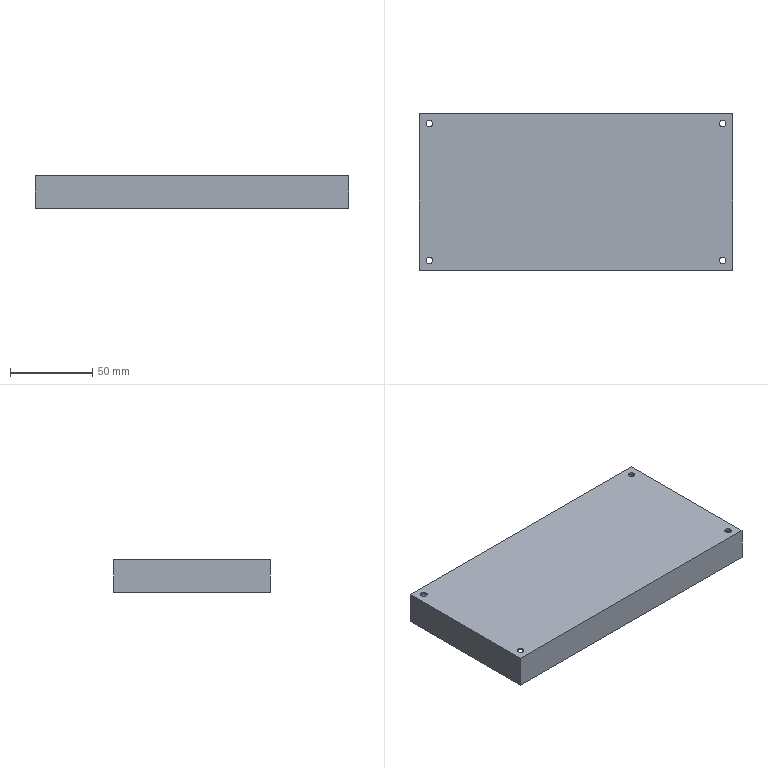Part | SolidWorks | features ICE 9, Extrusion 1, Shell 1 | 1 solid | 19 faces | box 190 x 95 x 20 mm | volume 28754 mm3 | plane 11 | cylinder 8 | commonest cylinder face diameters 4 x8
STEP:
#1=CARTESIAN_POINT('',(154.139,-3.375,19.));
#2=VERTEX_POINT('',#1);
#3=CARTESIAN_POINT('',(158.139,-3.375,19.));
#4=VERTEX_POINT('',#3);
#5=CARTESIAN_POINT('',(156.139,-3.375,19.));
#6=DIRECTION('',(0.,0.,1.));
#7=DIRECTION('',(1.,0.,0.));
#8=AXIS2_PLACEMENT_3D('',#5,#6,#7);
#9=CIRCLE('',#8,2.);
#10=EDGE_CURVE('',#2,#4,#9,.T.);
#11=ORIENTED_EDGE('',*,*,#10,.F.);
#12=CARTESIAN_POINT('',(154.139,-3.375,20.));
#13=VERTEX_POINT('',#12);
#14=CARTESIAN_POINT('',(154.139,-3.375,19.));
#15=DIRECTION('',(0.,0.,1.));
#16=VECTOR('',#15,1000.);
#17=LINE('',#14,#16);
#18=EDGE_CURVE('',#2,#13,#17,.T.);
#19=ORIENTED_EDGE('',*,*,#18,.T.);
#20=CARTESIAN_POINT('',(158.139,-3.375,20.));
#21=VERTEX_POINT('',#20);
#22=CARTESIAN_POINT('',(156.139,-3.375,20.));
#23=DIRECTION('',(0.,0.,1.));
#24=DIRECTION('',(1.,0.,0.));
#25=AXIS2_PLACEMENT_3D('',#22,#23,#24);
#26=CIRCLE('',#25,2.);
#27=EDGE_CURVE('',#13,#21,#26,.T.);
#28=ORIENTED_EDGE('',*,*,#27,.T.);
#29=CARTESIAN_POINT('',(158.139,-3.375,19.));
#30=DIRECTION('',(0.,0.,1.));
#31=VECTOR('',#30,1000.);
#32=LINE('',#29,#31);
#33=EDGE_CURVE('',#4,#21,#32,.T.);
#34=ORIENTED_EDGE('',*,*,#33,.F.);
#35=EDGE_LOOP('',(#11,#19,#28,#34));
#36=FACE_OUTER_BOUND('',#35,.T.);
#37=CARTESIAN_POINT('',(156.139,-3.375,19.));
#38=DIRECTION('',(0.,0.,1.));
#39=DIRECTION('',(1.,0.,0.));
#40=AXIS2_PLACEMENT_3D('',#37,#38,#39);
#41=CYLINDRICAL_SURFACE('',#40,2.);
#42=ADVANCED_FACE('',(#36),#41,.F.);
#43=CARTESIAN_POINT('',(154.139,79.625,19.));
#44=VERTEX_POINT('',#43);
#45=CARTESIAN_POINT('',(158.139,79.625,19.));
#46=VERTEX_POINT('',#45);
#47=CARTESIAN_POINT('',(156.139,79.625,19.));
#48=DIRECTION('',(0.,0.,1.));
#49=DIRECTION('',(1.,0.,0.));
#50=AXIS2_PLACEMENT_3D('',#47,#48,#49);
#51=CIRCLE('',#50,2.);
#52=EDGE_CURVE('',#44,#46,#51,.T.);
#53=ORIENTED_EDGE('',*,*,#52,.F.);
#54=CARTESIAN_POINT('',(154.139,79.625,20.));
#55=VERTEX_POINT('',#54);
#56=CARTESIAN_POINT('',(154.139,79.625,19.));
#57=DIRECTION('',(0.,0.,1.));
#58=VECTOR('',#57,1000.);
#59=LINE('',#56,#58);
#60=EDGE_CURVE('',#44,#55,#59,.T.);
#61=ORIENTED_EDGE('',*,*,#60,.T.);
#62=CARTESIAN_POINT('',(158.139,79.625,20.));
#63=VERTEX_POINT('',#62);
#64=CARTESIAN_POINT('',(156.139,79.625,20.));
#65=DIRECTION('',(0.,0.,1.));
#66=DIRECTION('',(1.,0.,0.));
#67=AXIS2_PLACEMENT_3D('',#64,#65,#66);
#68=CIRCLE('',#67,2.);
#69=EDGE_CURVE('',#55,#63,#68,.T.);
#70=ORIENTED_EDGE('',*,*,#69,.T.);
#71=CARTESIAN_POINT('',(158.139,79.625,19.));
#72=DIRECTION('',(0.,0.,1.));
#73=VECTOR('',#72,1000.);
#74=LINE('',#71,#73);
#75=EDGE_CURVE('',#46,#63,#74,.T.);
#76=ORIENTED_EDGE('',*,*,#75,.F.);
#77=EDGE_LOOP('',(#53,#61,#70,#76));
#78=FACE_OUTER_BOUND('',#77,.T.);
#79=CARTESIAN_POINT('',(156.139,79.625,19.));
#80=DIRECTION('',(0.,0.,1.));
#81=DIRECTION('',(1.,0.,0.));
#82=AXIS2_PLACEMENT_3D('',#79,#80,#81);
#83=CYLINDRICAL_SURFACE('',#82,2.);
#84=ADVANCED_FACE('',(#78),#83,.F.);
#85=CARTESIAN_POINT('',(-23.861,79.625,19.));
#86=VERTEX_POINT('',#85);
#87=CARTESIAN_POINT('',(-19.861,79.625,19.));
#88=VERTEX_POINT('',#87);
#89=CARTESIAN_POINT('',(-21.861,79.625,19.));
#90=DIRECTION('',(0.,0.,1.));
#91=DIRECTION('',(1.,0.,0.));
#92=AXIS2_PLACEMENT_3D('',#89,#90,#91);
#93=CIRCLE('',#92,2.);
#94=EDGE_CURVE('',#86,#88,#93,.T.);
#95=ORIENTED_EDGE('',*,*,#94,.F.);
#96=CARTESIAN_POINT('',(-23.861,79.625,20.));
#97=VERTEX_POINT('',#96);
#98=CARTESIAN_POINT('',(-23.861,79.625,19.));
#99=DIRECTION('',(0.,0.,1.));
#100=VECTOR('',#99,1000.);
#101=LINE('',#98,#100);
#102=EDGE_CURVE('',#86,#97,#101,.T.);
#103=ORIENTED_EDGE('',*,*,#102,.T.);
#104=CARTESIAN_POINT('',(-19.861,79.625,20.));
#105=VERTEX_POINT('',#104);
#106=CARTESIAN_POINT('',(-21.861,79.625,20.));
#107=DIRECTION('',(0.,0.,1.));
#108=DIRECTION('',(1.,0.,0.));
#109=AXIS2_PLACEMENT_3D('',#106,#107,#108);
#110=CIRCLE('',#109,2.);
#111=EDGE_CURVE('',#97,#105,#110,.T.);
#112=ORIENTED_EDGE('',*,*,#111,.T.);
#113=CARTESIAN_POINT('',(-19.861,79.625,19.));
#114=DIRECTION('',(0.,0.,1.));
#115=VECTOR('',#114,1000.);
#116=LINE('',#113,#115);
#117=EDGE_CURVE('',#88,#105,#116,.T.);
#118=ORIENTED_EDGE('',*,*,#117,.F.);
#119=EDGE_LOOP('',(#95,#103,#112,#118));
#120=FACE_OUTER_BOUND('',#119,.T.);
#121=CARTESIAN_POINT('',(-21.861,79.625,19.));
#122=DIRECTION('',(0.,0.,1.));
#123=DIRECTION('',(1.,0.,0.));
#124=AXIS2_PLACEMENT_3D('',#121,#122,#123);
#125=CYLINDRICAL_SURFACE('',#124,2.);
#126=ADVANCED_FACE('',(#120),#125,.F.);
#127=CARTESIAN_POINT('',(-23.861,-3.375,19.));
#128=VERTEX_POINT('',#127);
#129=CARTESIAN_POINT('',(-19.861,-3.375,19.));
#130=VERTEX_POINT('',#129);
#131=CARTESIAN_POINT('',(-21.861,-3.375,19.));
#132=DIRECTION('',(0.,0.,1.));
#133=DIRECTION('',(1.,0.,0.));
#134=AXIS2_PLACEMENT_3D('',#131,#132,#133);
#135=CIRCLE('',#134,2.);
#136=EDGE_CURVE('',#128,#130,#135,.T.);
#137=ORIENTED_EDGE('',*,*,#136,.F.);
#138=CARTESIAN_POINT('',(-23.861,-3.375,20.));
#139=VERTEX_POINT('',#138);
#140=CARTESIAN_POINT('',(-23.861,-3.375,19.));
#141=DIRECTION('',(0.,0.,1.));
#142=VECTOR('',#141,1000.);
#143=LINE('',#140,#142);
#144=EDGE_CURVE('',#128,#139,#143,.T.);
#145=ORIENTED_EDGE('',*,*,#144,.T.);
#146=CARTESIAN_POINT('',(-19.861,-3.375,20.));
#147=VERTEX_POINT('',#146);
#148=CARTESIAN_POINT('',(-21.861,-3.375,20.));
#149=DIRECTION('',(0.,0.,1.));
#150=DIRECTION('',(1.,0.,0.));
#151=AXIS2_PLACEMENT_3D('',#148,#149,#150);
#152=CIRCLE('',#151,2.);
#153=EDGE_CURVE('',#139,#147,#152,.T.);
#154=ORIENTED_EDGE('',*,*,#153,.T.);
#155=CARTESIAN_POINT('',(-19.861,-3.375,19.));
#156=DIRECTION('',(0.,0.,1.));
#157=VECTOR('',#156,1000.);
#158=LINE('',#155,#157);
#159=EDGE_CURVE('',#130,#147,#158,.T.);
#160=ORIENTED_EDGE('',*,*,#159,.F.);
#161=EDGE_LOOP('',(#137,#145,#154,#160));
#162=FACE_OUTER_BOUND('',#161,.T.);
#163=CARTESIAN_POINT('',(-21.861,-3.375,19.));
#164=DIRECTION('',(0.,0.,1.));
#165=DIRECTION('',(1.,0.,0.));
#166=AXIS2_PLACEMENT_3D('',#163,#164,#165);
#167=CYLINDRICAL_SURFACE('',#166,2.);
#168=ADVANCED_FACE('',(#162),#167,.F.);
#169=CARTESIAN_POINT('',(-27.861,-9.375,0.));
#170=VERTEX_POINT('',#169);
#171=CARTESIAN_POINT('',(162.139,-9.375,0.));
#172=VERTEX_POINT('',#171);
#173=CARTESIAN_POINT('',(-27.861,-9.375,0.));
#174=DIRECTION('',(1.,0.,0.));
#175=VECTOR('',#174,1000.);
#176=LINE('',#173,#175);
#177=EDGE_CURVE('',#170,#172,#176,.T.);
#178=ORIENTED_EDGE('',*,*,#177,.T.);
#179=CARTESIAN_POINT('',(162.139,-9.375,20.));
#180=VERTEX_POINT('',#179);
#181=CARTESIAN_POINT('',(162.139,-9.375,20.));
#182=DIRECTION('',(0.,0.,-1.));
#183=VECTOR('',#182,1000.);
#184=LINE('',#181,#183);
#185=EDGE_CURVE('',#180,#172,#184,.T.);
#186=ORIENTED_EDGE('',*,*,#185,.F.);
#187=CARTESIAN_POINT('',(-27.861,-9.375,20.));
#188=VERTEX_POINT('',#187);
#189=CARTESIAN_POINT('',(-27.861,-9.375,20.));
#190=DIRECTION('',(1.,0.,0.));
#191=VECTOR('',#190,1000.);
#192=LINE('',#189,#191);
#193=EDGE_CURVE('',#188,#180,#192,.T.);
#194=ORIENTED_EDGE('',*,*,#193,.F.);
#195=CARTESIAN_POINT('',(-27.861,-9.375,20.));
#196=DIRECTION('',(0.,0.,-1.));
#197=VECTOR('',#196,1000.);
#198=LINE('',#195,#197);
#199=EDGE_CURVE('',#188,#170,#198,.T.);
#200=ORIENTED_EDGE('',*,*,#199,.T.);
#201=EDGE_LOOP('',(#178,#186,#194,#200));
#202=FACE_OUTER_BOUND('',#201,.T.);
#203=CARTESIAN_POINT('',(-27.861,-9.375,20.));
#204=DIRECTION('',(0.,1.,0.));
#205=DIRECTION('',(0.,0.,1.));
#206=AXIS2_PLACEMENT_3D('',#203,#204,#205);
#207=PLANE('',#206);
#208=ADVANCED_FACE('',(#202),#207,.F.);
#209=CARTESIAN_POINT('',(-26.861,-8.375,19.));
#210=VERTEX_POINT('',#209);
#211=CARTESIAN_POINT('',(161.139,-8.375,19.));
#212=VERTEX_POINT('',#211);
#213=CARTESIAN_POINT('',(-27.861,-8.375,19.));
#214=DIRECTION('',(1.,0.,0.));
#215=VECTOR('',#214,1000.);
#216=LINE('',#213,#215);
#217=EDGE_CURVE('',#210,#212,#216,.T.);
#218=ORIENTED_EDGE('',*,*,#217,.T.);
#219=CARTESIAN_POINT('',(161.139,-8.375,0.));
#220=VERTEX_POINT('',#219);
#221=CARTESIAN_POINT('',(161.139,-8.375,20.));
#222=DIRECTION('',(0.,0.,-1.));
#223=VECTOR('',#222,1000.);
#224=LINE('',#221,#223);
#225=EDGE_CURVE('',#212,#220,#224,.T.);
#226=ORIENTED_EDGE('',*,*,#225,.T.);
#227=CARTESIAN_POINT('',(-26.861,-8.375,0.));
#228=VERTEX_POINT('',#227);
#229=CARTESIAN_POINT('',(-27.861,-8.375,0.));
#230=DIRECTION('',(1.,0.,0.));
#231=VECTOR('',#230,1000.);
#232=LINE('',#229,#231);
#233=EDGE_CURVE('',#228,#220,#232,.T.);
#234=ORIENTED_EDGE('',*,*,#233,.F.);
#235=CARTESIAN_POINT('',(-26.861,-8.375,20.));
#236=DIRECTION('',(0.,0.,-1.));
#237=VECTOR('',#236,1000.);
#238=LINE('',#235,#237);
#239=EDGE_CURVE('',#210,#228,#238,.T.);
#240=ORIENTED_EDGE('',*,*,#239,.F.);
#241=EDGE_LOOP('',(#218,#226,#234,#240));
#242=FACE_OUTER_BOUND('',#241,.T.);
#243=CARTESIAN_POINT('',(-27.861,-8.375,20.));
#244=DIRECTION('',(0.,1.,0.));
#245=DIRECTION('',(0.,0.,1.));
#246=AXIS2_PLACEMENT_3D('',#243,#244,#245);
#247=PLANE('',#246);
#248=ADVANCED_FACE('',(#242),#247,.T.);
#249=CARTESIAN_POINT('',(161.139,84.625,19.));
#250=VERTEX_POINT('',#249);
#251=CARTESIAN_POINT('',(-26.861,84.625,19.));
#252=VERTEX_POINT('',#251);
#253=CARTESIAN_POINT('',(-27.861,84.625,19.));
#254=DIRECTION('',(-1.,0.,0.));
#255=VECTOR('',#254,1000.);
#256=LINE('',#253,#255);
#257=EDGE_CURVE('',#250,#252,#256,.T.);
#258=ORIENTED_EDGE('',*,*,#257,.T.);
#259=CARTESIAN_POINT('',(-26.861,84.625,0.));
#260=VERTEX_POINT('',#259);
#261=CARTESIAN_POINT('',(-26.861,84.625,20.));
#262=DIRECTION('',(0.,0.,-1.));
#263=VECTOR('',#262,1000.);
#264=LINE('',#261,#263);
#265=EDGE_CURVE('',#252,#260,#264,.T.);
#266=ORIENTED_EDGE('',*,*,#265,.T.);
#267=CARTESIAN_POINT('',(161.139,84.625,0.));
#268=VERTEX_POINT('',#267);
#269=CARTESIAN_POINT('',(-27.861,84.625,0.));
#270=DIRECTION('',(-1.,0.,0.));
#271=VECTOR('',#270,1000.);
#272=LINE('',#269,#271);
#273=EDGE_CURVE('',#268,#260,#272,.T.);
#274=ORIENTED_EDGE('',*,*,#273,.F.);
#275=CARTESIAN_POINT('',(161.139,84.625,20.));
#276=DIRECTION('',(0.,0.,-1.));
#277=VECTOR('',#276,1000.);
#278=LINE('',#275,#277);
#279=EDGE_CURVE('',#250,#268,#278,.T.);
#280=ORIENTED_EDGE('',*,*,#279,.F.);
#281=EDGE_LOOP('',(#258,#266,#274,#280));
#282=FACE_OUTER_BOUND('',#281,.T.);
#283=CARTESIAN_POINT('',(-27.861,84.625,20.));
#284=DIRECTION('',(0.,-1.,0.));
#285=DIRECTION('',(0.,0.,-1.));
#286=AXIS2_PLACEMENT_3D('',#283,#284,#285);
#287=PLANE('',#286);
#288=ADVANCED_FACE('',(#282),#287,.T.);
#289=CARTESIAN_POINT('',(162.139,85.625,0.));
#290=VERTEX_POINT('',#289);
#291=CARTESIAN_POINT('',(-27.861,85.625,0.));
#292=VERTEX_POINT('',#291);
#293=CARTESIAN_POINT('',(-27.861,85.625,0.));
#294=DIRECTION('',(-1.,0.,0.));
#295=VECTOR('',#294,1000.);
#296=LINE('',#293,#295);
#297=EDGE_CURVE('',#290,#292,#296,.T.);
#298=ORIENTED_EDGE('',*,*,#297,.T.);
#299=CARTESIAN_POINT('',(-27.861,85.625,20.));
#300=VERTEX_POINT('',#299);
#301=CARTESIAN_POINT('',(-27.861,85.625,20.));
#302=DIRECTION('',(0.,0.,-1.));
#303=VECTOR('',#302,1000.);
#304=LINE('',#301,#303);
#305=EDGE_CURVE('',#300,#292,#304,.T.);
#306=ORIENTED_EDGE('',*,*,#305,.F.);
#307=CARTESIAN_POINT('',(162.139,85.625,20.));
#308=VERTEX_POINT('',#307);
#309=CARTESIAN_POINT('',(-27.861,85.625,20.));
#310=DIRECTION('',(-1.,0.,0.));
#311=VECTOR('',#310,1000.);
#312=LINE('',#309,#311);
#313=EDGE_CURVE('',#308,#300,#312,.T.);
#314=ORIENTED_EDGE('',*,*,#313,.F.);
#315=CARTESIAN_POINT('',(162.139,85.625,20.));
#316=DIRECTION('',(0.,0.,-1.));
#317=VECTOR('',#316,1000.);
#318=LINE('',#315,#317);
#319=EDGE_CURVE('',#308,#290,#318,.T.);
#320=ORIENTED_EDGE('',*,*,#319,.T.);
#321=EDGE_LOOP('',(#298,#306,#314,#320));
#322=FACE_OUTER_BOUND('',#321,.T.);
#323=CARTESIAN_POINT('',(-27.861,85.625,20.));
#324=DIRECTION('',(0.,-1.,0.));
#325=DIRECTION('',(0.,0.,-1.));
#326=AXIS2_PLACEMENT_3D('',#323,#324,#325);
#327=PLANE('',#326);
#328=ADVANCED_FACE('',(#322),#327,.F.);
#329=CARTESIAN_POINT('',(-27.861,85.625,0.));
#330=DIRECTION('',(0.,-1.,0.));
#331=VECTOR('',#330,1000.);
#332=LINE('',#329,#331);
#333=EDGE_CURVE('',#292,#170,#332,.T.);
#334=ORIENTED_EDGE('',*,*,#333,.T.);
#335=ORIENTED_EDGE('',*,*,#199,.F.);
#336=CARTESIAN_POINT('',(-27.861,85.625,20.));
#337=DIRECTION('',(0.,-1.,0.));
#338=VECTOR('',#337,1000.);
#339=LINE('',#336,#338);
#340=EDGE_CURVE('',#300,#188,#339,.T.);
#341=ORIENTED_EDGE('',*,*,#340,.F.);
#342=ORIENTED_EDGE('',*,*,#305,.T.);
#343=EDGE_LOOP('',(#334,#335,#341,#342));
#344=FACE_OUTER_BOUND('',#343,.T.);
#345=CARTESIAN_POINT('',(-27.861,85.625,20.));
#346=DIRECTION('',(1.,0.,0.));
#347=DIRECTION('',(0.,1.,0.));
#348=AXIS2_PLACEMENT_3D('',#345,#346,#347);
#349=PLANE('',#348);
#350=ADVANCED_FACE('',(#344),#349,.F.);
#351=CARTESIAN_POINT('',(162.139,85.625,0.));
#352=DIRECTION('',(0.,1.,0.));
#353=VECTOR('',#352,1000.);
#354=LINE('',#351,#353);
#355=EDGE_CURVE('',#172,#290,#354,.T.);
#356=ORIENTED_EDGE('',*,*,#355,.T.);
#357=ORIENTED_EDGE('',*,*,#319,.F.);
#358=CARTESIAN_POINT('',(162.139,85.625,20.));
#359=DIRECTION('',(0.,1.,0.));
#360=VECTOR('',#359,1000.);
#361=LINE('',#358,#360);
#362=EDGE_CURVE('',#180,#308,#361,.T.);
#363=ORIENTED_EDGE('',*,*,#362,.F.);
#364=ORIENTED_EDGE('',*,*,#185,.T.);
#365=EDGE_LOOP('',(#356,#357,#363,#364));
#366=FACE_OUTER_BOUND('',#365,.T.);
#367=CARTESIAN_POINT('',(162.139,85.625,20.));
#368=DIRECTION('',(-1.,0.,0.));
#369=DIRECTION('',(0.,0.,1.));
#370=AXIS2_PLACEMENT_3D('',#367,#368,#369);
#371=PLANE('',#370);
#372=ADVANCED_FACE('',(#366),#371,.F.);
#373=CARTESIAN_POINT('',(156.139,-3.375,20.));
#374=DIRECTION('',(0.,0.,1.));
#375=DIRECTION('',(1.,0.,0.));
#376=AXIS2_PLACEMENT_3D('',#373,#374,#375);
#377=CIRCLE('',#376,2.);
#378=EDGE_CURVE('',#21,#13,#377,.T.);
#379=ORIENTED_EDGE('',*,*,#378,.F.);
#380=ORIENTED_EDGE('',*,*,#27,.F.);
#381=EDGE_LOOP('',(#379,#380));
#382=FACE_BOUND('',#381,.T.);
#383=CARTESIAN_POINT('',(156.139,79.625,20.));
#384=DIRECTION('',(0.,0.,1.));
#385=DIRECTION('',(1.,0.,0.));
#386=AXIS2_PLACEMENT_3D('',#383,#384,#385);
#387=CIRCLE('',#386,2.);
#388=EDGE_CURVE('',#63,#55,#387,.T.);
#389=ORIENTED_EDGE('',*,*,#388,.F.);
#390=ORIENTED_EDGE('',*,*,#69,.F.);
#391=EDGE_LOOP('',(#389,#390));
#392=FACE_BOUND('',#391,.T.);
#393=CARTESIAN_POINT('',(-21.861,79.625,20.));
#394=DIRECTION('',(0.,0.,1.));
#395=DIRECTION('',(1.,0.,0.));
#396=AXIS2_PLACEMENT_3D('',#393,#394,#395);
#397=CIRCLE('',#396,2.);
#398=EDGE_CURVE('',#105,#97,#397,.T.);
#399=ORIENTED_EDGE('',*,*,#398,.F.);
#400=ORIENTED_EDGE('',*,*,#111,.F.);
#401=EDGE_LOOP('',(#399,#400));
#402=FACE_BOUND('',#401,.T.);
#403=CARTESIAN_POINT('',(-21.861,-3.375,20.));
#404=DIRECTION('',(0.,0.,1.));
#405=DIRECTION('',(1.,0.,0.));
#406=AXIS2_PLACEMENT_3D('',#403,#404,#405);
#407=CIRCLE('',#406,2.);
#408=EDGE_CURVE('',#147,#139,#407,.T.);
#409=ORIENTED_EDGE('',*,*,#408,.F.);
#410=ORIENTED_EDGE('',*,*,#153,.F.);
#411=EDGE_LOOP('',(#409,#410));
#412=FACE_BOUND('',#411,.T.);
#413=ORIENTED_EDGE('',*,*,#340,.T.);
#414=ORIENTED_EDGE('',*,*,#193,.T.);
#415=ORIENTED_EDGE('',*,*,#362,.T.);
#416=ORIENTED_EDGE('',*,*,#313,.T.);
#417=EDGE_LOOP('',(#413,#414,#415,#416));
#418=FACE_OUTER_BOUND('',#417,.T.);
#419=CARTESIAN_POINT('',(0.,0.,20.));
#420=DIRECTION('',(0.,0.,1.));
#421=DIRECTION('',(1.,0.,0.));
#422=AXIS2_PLACEMENT_3D('',#419,#420,#421);
#423=PLANE('',#422);
#424=ADVANCED_FACE('',(#382,#392,#402,#412,#418),#423,.T.);
#425=ORIENTED_EDGE('',*,*,#273,.T.);
#426=CARTESIAN_POINT('',(-26.861,85.625,0.));
#427=DIRECTION('',(0.,-1.,0.));
#428=VECTOR('',#427,1000.);
#429=LINE('',#426,#428);
#430=EDGE_CURVE('',#260,#228,#429,.T.);
#431=ORIENTED_EDGE('',*,*,#430,.T.);
#432=ORIENTED_EDGE('',*,*,#233,.T.);
#433=CARTESIAN_POINT('',(161.139,85.625,0.));
#434=DIRECTION('',(0.,1.,0.));
#435=VECTOR('',#434,1000.);
#436=LINE('',#433,#435);
#437=EDGE_CURVE('',#220,#268,#436,.T.);
#438=ORIENTED_EDGE('',*,*,#437,.T.);
#439=EDGE_LOOP('',(#425,#431,#432,#438));
#440=FACE_BOUND('',#439,.T.);
#441=ORIENTED_EDGE('',*,*,#333,.F.);
#442=ORIENTED_EDGE('',*,*,#297,.F.);
#443=ORIENTED_EDGE('',*,*,#355,.F.);
#444=ORIENTED_EDGE('',*,*,#177,.F.);
#445=EDGE_LOOP('',(#441,#442,#443,#444));
#446=FACE_OUTER_BOUND('',#445,.T.);
#447=CARTESIAN_POINT('',(0.,0.,0.));
#448=DIRECTION('',(0.,0.,1.));
#449=DIRECTION('',(1.,0.,0.));
#450=AXIS2_PLACEMENT_3D('',#447,#448,#449);
#451=PLANE('',#450);
#452=ADVANCED_FACE('',(#440,#446),#451,.F.);
#453=ORIENTED_EDGE('',*,*,#430,.F.);
#454=ORIENTED_EDGE('',*,*,#265,.F.);
#455=CARTESIAN_POINT('',(-26.861,85.625,19.));
#456=DIRECTION('',(0.,-1.,0.));
#457=VECTOR('',#456,1000.);
#458=LINE('',#455,#457);
#459=EDGE_CURVE('',#252,#210,#458,.T.);
#460=ORIENTED_EDGE('',*,*,#459,.T.);
#461=ORIENTED_EDGE('',*,*,#239,.T.);
#462=EDGE_LOOP('',(#453,#454,#460,#461));
#463=FACE_OUTER_BOUND('',#462,.T.);
#464=CARTESIAN_POINT('',(-26.861,85.625,20.));
#465=DIRECTION('',(1.,0.,0.));
#466=DIRECTION('',(0.,1.,0.));
#467=AXIS2_PLACEMENT_3D('',#464,#465,#466);
#468=PLANE('',#467);
#469=ADVANCED_FACE('',(#463),#468,.T.);
#470=ORIENTED_EDGE('',*,*,#437,.F.);
#471=ORIENTED_EDGE('',*,*,#225,.F.);
#472=CARTESIAN_POINT('',(161.139,85.625,19.));
#473=DIRECTION('',(0.,1.,0.));
#474=VECTOR('',#473,1000.);
#475=LINE('',#472,#474);
#476=EDGE_CURVE('',#212,#250,#475,.T.);
#477=ORIENTED_EDGE('',*,*,#476,.T.);
#478=ORIENTED_EDGE('',*,*,#279,.T.);
#479=EDGE_LOOP('',(#470,#471,#477,#478));
#480=FACE_OUTER_BOUND('',#479,.T.);
#481=CARTESIAN_POINT('',(161.139,85.625,20.));
#482=DIRECTION('',(-1.,0.,0.));
#483=DIRECTION('',(0.,0.,1.));
#484=AXIS2_PLACEMENT_3D('',#481,#482,#483);
#485=PLANE('',#484);
#486=ADVANCED_FACE('',(#480),#485,.T.);
#487=CARTESIAN_POINT('',(156.139,-3.375,19.));
#488=DIRECTION('',(0.,0.,1.));
#489=DIRECTION('',(1.,0.,0.));
#490=AXIS2_PLACEMENT_3D('',#487,#488,#489);
#491=CIRCLE('',#490,2.);
#492=EDGE_CURVE('',#4,#2,#491,.T.);
#493=ORIENTED_EDGE('',*,*,#492,.T.);
#494=ORIENTED_EDGE('',*,*,#10,.T.);
#495=EDGE_LOOP('',(#493,#494));
#496=FACE_BOUND('',#495,.T.);
#497=CARTESIAN_POINT('',(156.139,79.625,19.));
#498=DIRECTION('',(0.,0.,1.));
#499=DIRECTION('',(1.,0.,0.));
#500=AXIS2_PLACEMENT_3D('',#497,#498,#499);
#501=CIRCLE('',#500,2.);
#502=EDGE_CURVE('',#46,#44,#501,.T.);
#503=ORIENTED_EDGE('',*,*,#502,.T.);
#504=ORIENTED_EDGE('',*,*,#52,.T.);
#505=EDGE_LOOP('',(#503,#504));
#506=FACE_BOUND('',#505,.T.);
#507=CARTESIAN_POINT('',(-21.861,79.625,19.));
#508=DIRECTION('',(0.,0.,1.));
#509=DIRECTION('',(1.,0.,0.));
#510=AXIS2_PLACEMENT_3D('',#507,#508,#509);
#511=CIRCLE('',#510,2.);
#512=EDGE_CURVE('',#88,#86,#511,.T.);
#513=ORIENTED_EDGE('',*,*,#512,.T.);
#514=ORIENTED_EDGE('',*,*,#94,.T.);
#515=EDGE_LOOP('',(#513,#514));
#516=FACE_BOUND('',#515,.T.);
#517=CARTESIAN_POINT('',(-21.861,-3.375,19.));
#518=DIRECTION('',(0.,0.,1.));
#519=DIRECTION('',(1.,0.,0.));
#520=AXIS2_PLACEMENT_3D('',#517,#518,#519);
#521=CIRCLE('',#520,2.);
#522=EDGE_CURVE('',#130,#128,#521,.T.);
#523=ORIENTED_EDGE('',*,*,#522,.T.);
#524=ORIENTED_EDGE('',*,*,#136,.T.);
#525=EDGE_LOOP('',(#523,#524));
#526=FACE_BOUND('',#525,.T.);
#527=ORIENTED_EDGE('',*,*,#459,.F.);
#528=ORIENTED_EDGE('',*,*,#257,.F.);
#529=ORIENTED_EDGE('',*,*,#476,.F.);
#530=ORIENTED_EDGE('',*,*,#217,.F.);
#531=EDGE_LOOP('',(#527,#528,#529,#530));
#532=FACE_OUTER_BOUND('',#531,.T.);
#533=CARTESIAN_POINT('',(0.,0.,19.));
#534=DIRECTION('',(0.,0.,1.));
#535=DIRECTION('',(1.,0.,0.));
#536=AXIS2_PLACEMENT_3D('',#533,#534,#535);
#537=PLANE('',#536);
#538=ADVANCED_FACE('',(#496,#506,#516,#526,#532),#537,.F.);
#539=ORIENTED_EDGE('',*,*,#144,.F.);
#540=ORIENTED_EDGE('',*,*,#522,.F.);
#541=ORIENTED_EDGE('',*,*,#159,.T.);
#542=ORIENTED_EDGE('',*,*,#408,.T.);
#543=EDGE_LOOP('',(#539,#540,#541,#542));
#544=FACE_OUTER_BOUND('',#543,.T.);
#545=CARTESIAN_POINT('',(-21.861,-3.375,19.));
#546=DIRECTION('',(0.,0.,1.));
#547=DIRECTION('',(1.,0.,0.));
#548=AXIS2_PLACEMENT_3D('',#545,#546,#547);
#549=CYLINDRICAL_SURFACE('',#548,2.);
#550=ADVANCED_FACE('',(#544),#549,.F.);
#551=ORIENTED_EDGE('',*,*,#102,.F.);
#552=ORIENTED_EDGE('',*,*,#512,.F.);
#553=ORIENTED_EDGE('',*,*,#117,.T.);
#554=ORIENTED_EDGE('',*,*,#398,.T.);
#555=EDGE_LOOP('',(#551,#552,#553,#554));
#556=FACE_OUTER_BOUND('',#555,.T.);
#557=CARTESIAN_POINT('',(-21.861,79.625,19.));
#558=DIRECTION('',(0.,0.,1.));
#559=DIRECTION('',(1.,0.,0.));
#560=AXIS2_PLACEMENT_3D('',#557,#558,#559);
#561=CYLINDRICAL_SURFACE('',#560,2.);
#562=ADVANCED_FACE('',(#556),#561,.F.);
#563=ORIENTED_EDGE('',*,*,#60,.F.);
#564=ORIENTED_EDGE('',*,*,#502,.F.);
#565=ORIENTED_EDGE('',*,*,#75,.T.);
#566=ORIENTED_EDGE('',*,*,#388,.T.);
#567=EDGE_LOOP('',(#563,#564,#565,#566));
#568=FACE_OUTER_BOUND('',#567,.T.);
#569=CARTESIAN_POINT('',(156.139,79.625,19.));
#570=DIRECTION('',(0.,0.,1.));
#571=DIRECTION('',(1.,0.,0.));
#572=AXIS2_PLACEMENT_3D('',#569,#570,#571);
#573=CYLINDRICAL_SURFACE('',#572,2.);
#574=ADVANCED_FACE('',(#568),#573,.F.);
#575=ORIENTED_EDGE('',*,*,#18,.F.);
#576=ORIENTED_EDGE('',*,*,#492,.F.);
#577=ORIENTED_EDGE('',*,*,#33,.T.);
#578=ORIENTED_EDGE('',*,*,#378,.T.);
#579=EDGE_LOOP('',(#575,#576,#577,#578));
#580=FACE_OUTER_BOUND('',#579,.T.);
#581=CARTESIAN_POINT('',(156.139,-3.375,19.));
#582=DIRECTION('',(0.,0.,1.));
#583=DIRECTION('',(1.,0.,0.));
#584=AXIS2_PLACEMENT_3D('',#581,#582,#583);
#585=CYLINDRICAL_SURFACE('',#584,2.);
#586=ADVANCED_FACE('',(#580),#585,.F.);
#587=CLOSED_SHELL('',(#42,#84,#126,#168,#208,#248,#288,#328,#350,#372,#424,#452,#469,#486,#538,#550,#562,#574,#586));
#588=MANIFOLD_SOLID_BREP('',#587);
#589=CARTESIAN_POINT('',(0.,0.,0.));
#590=DIRECTION('',(0.,0.,1.));
#591=DIRECTION('',(1.,0.,0.));
#592=AXIS2_PLACEMENT_3D('',#589,#590,#591);
#593=(LENGTH_UNIT()NAMED_UNIT(*)SI_UNIT(.MILLI.,.METRE.));
#594=UNCERTAINTY_MEASURE_WITH_UNIT(LENGTH_MEASURE(0.00001),#593,'','');
#595=(NAMED_UNIT(*)PLANE_ANGLE_UNIT()SI_UNIT($,.RADIAN.));
#596=(NAMED_UNIT(*)SI_UNIT($,.STERADIAN.)SOLID_ANGLE_UNIT());
#597=(GEOMETRIC_REPRESENTATION_CONTEXT(3)GLOBAL_UNCERTAINTY_ASSIGNED_CONTEXT((#594))GLOBAL_UNIT_ASSIGNED_CONTEXT((#593,#595,#596))REPRESENTATION_CONTEXT('',''));
#598=ADVANCED_BREP_SHAPE_REPRESENTATION('',(#588,#592),#597);